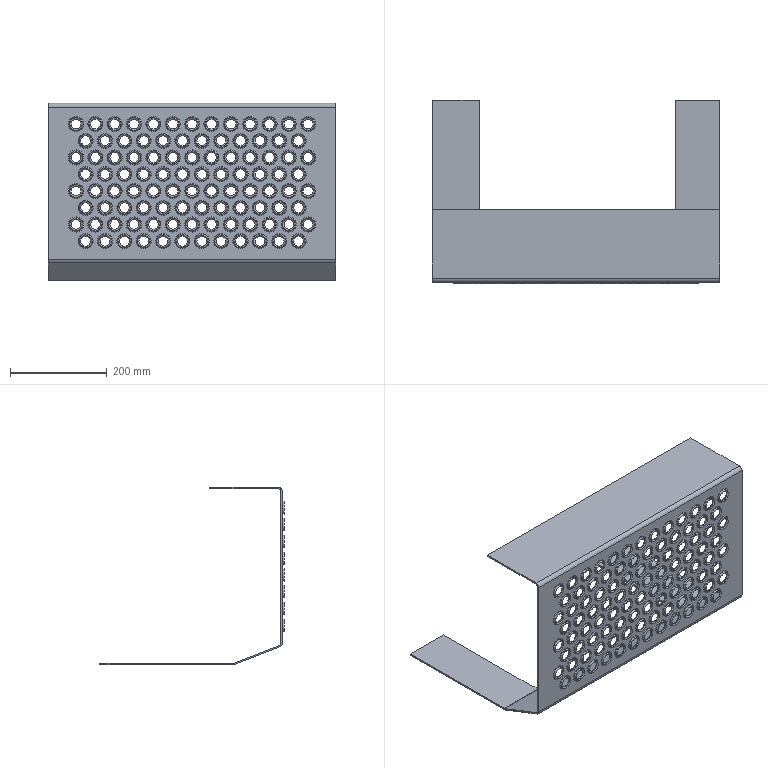Part | SolidWorks | features FormToolInstance 2, FlatPattern 1, ICE 1, SMBaseFlange 1, SheetMetal 1 | 1 solid | 1040 faces | box 593.5 x 380.4 x 367 mm | volume 1180890 mm3 | cone 600 | torus 400 | plane 30 | cylinder 8 | spline 2 | commonest cylinder face diameters 10 x3 16.4 x3 40 x2